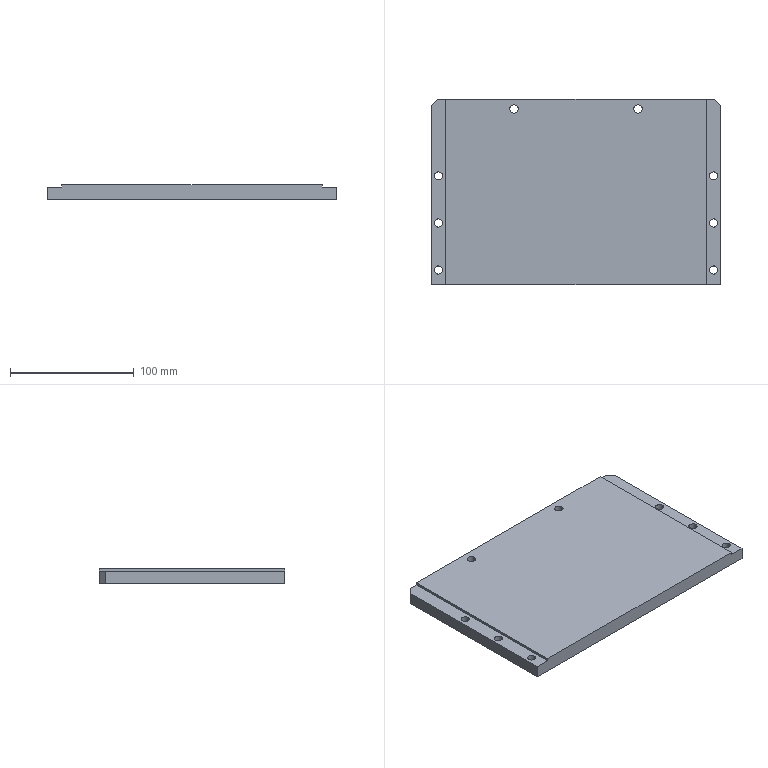Part | STEP file | 0228_208_Plate | 1 solid | 28 faces | box 234 x 150 x 12 mm | volume 410826 mm3 | cylinder 16 | plane 12 | commonest cylinder face diameters 6.6 x12 6.8 x4